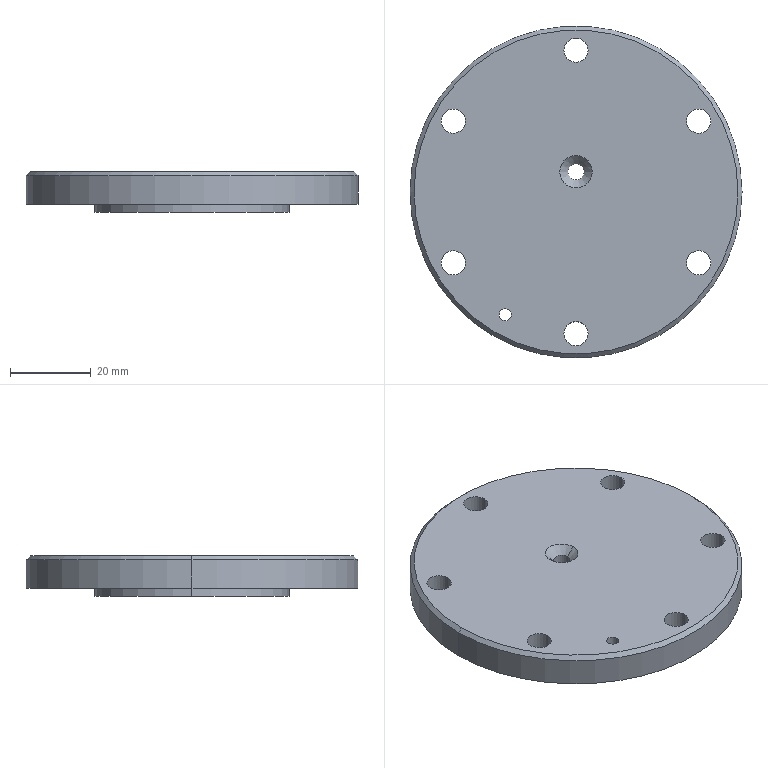Part | SolidWorks | features Chamfer 2, ICE 1, Revolution 1 | 1 solid | 27 faces | box 82 x 82 x 10 mm | volume 44167 mm3 | cylinder 20 | cone 4 | plane 3 | commonest cylinder face diameters 6 x12 3 x2 4 x2 48 x2 82 x2
STEP:
#1=CARTESIAN_POINT('',(-2.,5.,8.));
#2=VERTEX_POINT('',#1);
#3=CARTESIAN_POINT('',(2.,5.,8.));
#4=VERTEX_POINT('',#3);
#5=CARTESIAN_POINT('',(0.,5.,8.));
#6=DIRECTION('',(0.,0.,1.));
#7=DIRECTION('',(-1.,0.,0.));
#8=AXIS2_PLACEMENT_3D('',#5,#6,#7);
#9=CIRCLE('',#8,2.);
#10=EDGE_CURVE('',#2,#4,#9,.T.);
#11=ORIENTED_EDGE('',*,*,#10,.F.);
#12=CARTESIAN_POINT('',(-4.,5.,10.));
#13=VERTEX_POINT('',#12);
#14=CARTESIAN_POINT('',(-4.,5.,10.));
#15=DIRECTION('',(-0.7071,0.,0.7071));
#16=VECTOR('',#15,1000.);
#17=LINE('',#14,#16);
#18=EDGE_CURVE('',#2,#13,#17,.T.);
#19=ORIENTED_EDGE('',*,*,#18,.T.);
#20=CARTESIAN_POINT('',(4.,5.,10.));
#21=VERTEX_POINT('',#20);
#22=CARTESIAN_POINT('',(0.,5.,10.));
#23=DIRECTION('',(0.,0.,-1.));
#24=DIRECTION('',(-1.,0.,0.));
#25=AXIS2_PLACEMENT_3D('',#22,#23,#24);
#26=CIRCLE('',#25,4.);
#27=EDGE_CURVE('',#21,#13,#26,.T.);
#28=ORIENTED_EDGE('',*,*,#27,.F.);
#29=CARTESIAN_POINT('',(4.,5.,10.));
#30=DIRECTION('',(0.7071,0.,0.7071));
#31=VECTOR('',#30,1000.);
#32=LINE('',#29,#31);
#33=EDGE_CURVE('',#4,#21,#32,.T.);
#34=ORIENTED_EDGE('',*,*,#33,.F.);
#35=EDGE_LOOP('',(#11,#19,#28,#34));
#36=FACE_OUTER_BOUND('',#35,.T.);
#37=CARTESIAN_POINT('',(0.,5.,10.));
#38=DIRECTION('',(0.,0.,1.));
#39=DIRECTION('',(1.,0.,0.));
#40=AXIS2_PLACEMENT_3D('',#37,#38,#39);
#41=CONICAL_SURFACE('',#40,4.,0.7854);
#42=ADVANCED_FACE('',(#36),#41,.F.);
#43=CARTESIAN_POINT('',(40.,0.,10.));
#44=VERTEX_POINT('',#43);
#45=CARTESIAN_POINT('',(-40.,0.,10.));
#46=VERTEX_POINT('',#45);
#47=CARTESIAN_POINT('',(0.,0.,10.));
#48=DIRECTION('',(0.,0.,1.));
#49=DIRECTION('',(-1.,0.,0.));
#50=AXIS2_PLACEMENT_3D('',#47,#48,#49);
#51=CIRCLE('',#50,40.);
#52=EDGE_CURVE('',#44,#46,#51,.T.);
#53=ORIENTED_EDGE('',*,*,#52,.F.);
#54=CARTESIAN_POINT('',(41.,0.,9.));
#55=VERTEX_POINT('',#54);
#56=CARTESIAN_POINT('',(40.,0.,10.));
#57=DIRECTION('',(0.7071,0.,-0.7071));
#58=VECTOR('',#57,1000.);
#59=LINE('',#56,#58);
#60=EDGE_CURVE('',#44,#55,#59,.T.);
#61=ORIENTED_EDGE('',*,*,#60,.T.);
#62=CARTESIAN_POINT('',(-41.,0.,9.));
#63=VERTEX_POINT('',#62);
#64=CARTESIAN_POINT('',(0.,0.,9.));
#65=DIRECTION('',(0.,0.,-1.));
#66=DIRECTION('',(-1.,0.,0.));
#67=AXIS2_PLACEMENT_3D('',#64,#65,#66);
#68=CIRCLE('',#67,41.);
#69=EDGE_CURVE('',#63,#55,#68,.T.);
#70=ORIENTED_EDGE('',*,*,#69,.F.);
#71=CARTESIAN_POINT('',(-40.,0.,10.));
#72=DIRECTION('',(-0.7071,0.,-0.7071));
#73=VECTOR('',#72,1000.);
#74=LINE('',#71,#73);
#75=EDGE_CURVE('',#46,#63,#74,.T.);
#76=ORIENTED_EDGE('',*,*,#75,.F.);
#77=EDGE_LOOP('',(#53,#61,#70,#76));
#78=FACE_OUTER_BOUND('',#77,.T.);
#79=CARTESIAN_POINT('',(0.,0.,10.));
#80=DIRECTION('',(0.,0.,-1.));
#81=DIRECTION('',(-1.,0.,0.));
#82=AXIS2_PLACEMENT_3D('',#79,#80,#81);
#83=CONICAL_SURFACE('',#82,40.,0.7854);
#84=ADVANCED_FACE('',(#78),#83,.T.);
#85=CARTESIAN_POINT('',(3.,35.,2.));
#86=VERTEX_POINT('',#85);
#87=CARTESIAN_POINT('',(-3.,35.,2.));
#88=VERTEX_POINT('',#87);
#89=CARTESIAN_POINT('',(0.,35.,2.));
#90=DIRECTION('',(0.,0.,-1.));
#91=DIRECTION('',(1.,0.,0.));
#92=AXIS2_PLACEMENT_3D('',#89,#90,#91);
#93=CIRCLE('',#92,3.);
#94=EDGE_CURVE('',#86,#88,#93,.T.);
#95=ORIENTED_EDGE('',*,*,#94,.T.);
#96=CARTESIAN_POINT('',(-3.,35.,10.));
#97=VERTEX_POINT('',#96);
#98=CARTESIAN_POINT('',(-3.,35.,-8.));
#99=DIRECTION('',(0.,0.,1.));
#100=VECTOR('',#99,1000.);
#101=LINE('',#98,#100);
#102=EDGE_CURVE('',#88,#97,#101,.T.);
#103=ORIENTED_EDGE('',*,*,#102,.T.);
#104=CARTESIAN_POINT('',(3.,35.,10.));
#105=VERTEX_POINT('',#104);
#106=CARTESIAN_POINT('',(0.,35.,10.));
#107=DIRECTION('',(0.,0.,-1.));
#108=DIRECTION('',(-1.,0.,0.));
#109=AXIS2_PLACEMENT_3D('',#106,#107,#108);
#110=CIRCLE('',#109,3.);
#111=EDGE_CURVE('',#105,#97,#110,.T.);
#112=ORIENTED_EDGE('',*,*,#111,.F.);
#113=CARTESIAN_POINT('',(3.,35.,-8.));
#114=DIRECTION('',(0.,0.,1.));
#115=VECTOR('',#114,1000.);
#116=LINE('',#113,#115);
#117=EDGE_CURVE('',#86,#105,#116,.T.);
#118=ORIENTED_EDGE('',*,*,#117,.F.);
#119=EDGE_LOOP('',(#95,#103,#112,#118));
#120=FACE_OUTER_BOUND('',#119,.T.);
#121=CARTESIAN_POINT('',(0.,35.,-8.));
#122=DIRECTION('',(0.,0.,1.));
#123=DIRECTION('',(1.,0.,0.));
#124=AXIS2_PLACEMENT_3D('',#121,#122,#123);
#125=CYLINDRICAL_SURFACE('',#124,3.);
#126=ADVANCED_FACE('',(#120),#125,.F.);
#127=CARTESIAN_POINT('',(33.311,17.5,2.));
#128=VERTEX_POINT('',#127);
#129=CARTESIAN_POINT('',(27.311,17.5,2.));
#130=VERTEX_POINT('',#129);
#131=CARTESIAN_POINT('',(30.311,17.5,2.));
#132=DIRECTION('',(0.,0.,-1.));
#133=DIRECTION('',(1.,0.,0.));
#134=AXIS2_PLACEMENT_3D('',#131,#132,#133);
#135=CIRCLE('',#134,3.);
#136=EDGE_CURVE('',#128,#130,#135,.T.);
#137=ORIENTED_EDGE('',*,*,#136,.T.);
#138=CARTESIAN_POINT('',(27.311,17.5,10.));
#139=VERTEX_POINT('',#138);
#140=CARTESIAN_POINT('',(27.311,17.5,-8.));
#141=DIRECTION('',(0.,0.,1.));
#142=VECTOR('',#141,1000.);
#143=LINE('',#140,#142);
#144=EDGE_CURVE('',#130,#139,#143,.T.);
#145=ORIENTED_EDGE('',*,*,#144,.T.);
#146=CARTESIAN_POINT('',(33.311,17.5,10.));
#147=VERTEX_POINT('',#146);
#148=CARTESIAN_POINT('',(30.311,17.5,10.));
#149=DIRECTION('',(0.,0.,-1.));
#150=DIRECTION('',(-1.,0.,0.));
#151=AXIS2_PLACEMENT_3D('',#148,#149,#150);
#152=CIRCLE('',#151,3.);
#153=EDGE_CURVE('',#147,#139,#152,.T.);
#154=ORIENTED_EDGE('',*,*,#153,.F.);
#155=CARTESIAN_POINT('',(33.311,17.5,-8.));
#156=DIRECTION('',(0.,0.,1.));
#157=VECTOR('',#156,1000.);
#158=LINE('',#155,#157);
#159=EDGE_CURVE('',#128,#147,#158,.T.);
#160=ORIENTED_EDGE('',*,*,#159,.F.);
#161=EDGE_LOOP('',(#137,#145,#154,#160));
#162=FACE_OUTER_BOUND('',#161,.T.);
#163=CARTESIAN_POINT('',(30.311,17.5,-8.));
#164=DIRECTION('',(0.,0.,1.));
#165=DIRECTION('',(1.,0.,0.));
#166=AXIS2_PLACEMENT_3D('',#163,#164,#165);
#167=CYLINDRICAL_SURFACE('',#166,3.);
#168=ADVANCED_FACE('',(#162),#167,.F.);
#169=CARTESIAN_POINT('',(-16.,-30.311,2.));
#170=VERTEX_POINT('',#169);
#171=CARTESIAN_POINT('',(-19.,-30.311,2.));
#172=VERTEX_POINT('',#171);
#173=CARTESIAN_POINT('',(-17.5,-30.311,2.));
#174=DIRECTION('',(0.,0.,-1.));
#175=DIRECTION('',(1.,0.,0.));
#176=AXIS2_PLACEMENT_3D('',#173,#174,#175);
#177=CIRCLE('',#176,1.5);
#178=EDGE_CURVE('',#170,#172,#177,.T.);
#179=ORIENTED_EDGE('',*,*,#178,.T.);
#180=CARTESIAN_POINT('',(-19.,-30.311,10.));
#181=VERTEX_POINT('',#180);
#182=CARTESIAN_POINT('',(-19.,-30.311,-8.));
#183=DIRECTION('',(0.,0.,1.));
#184=VECTOR('',#183,1000.);
#185=LINE('',#182,#184);
#186=EDGE_CURVE('',#172,#181,#185,.T.);
#187=ORIENTED_EDGE('',*,*,#186,.T.);
#188=CARTESIAN_POINT('',(-16.,-30.311,10.));
#189=VERTEX_POINT('',#188);
#190=CARTESIAN_POINT('',(-17.5,-30.311,10.));
#191=DIRECTION('',(0.,0.,-1.));
#192=DIRECTION('',(-1.,0.,0.));
#193=AXIS2_PLACEMENT_3D('',#190,#191,#192);
#194=CIRCLE('',#193,1.5);
#195=EDGE_CURVE('',#189,#181,#194,.T.);
#196=ORIENTED_EDGE('',*,*,#195,.F.);
#197=CARTESIAN_POINT('',(-16.,-30.311,-8.));
#198=DIRECTION('',(0.,0.,1.));
#199=VECTOR('',#198,1000.);
#200=LINE('',#197,#199);
#201=EDGE_CURVE('',#170,#189,#200,.T.);
#202=ORIENTED_EDGE('',*,*,#201,.F.);
#203=EDGE_LOOP('',(#179,#187,#196,#202));
#204=FACE_OUTER_BOUND('',#203,.T.);
#205=CARTESIAN_POINT('',(-17.5,-30.311,-8.));
#206=DIRECTION('',(0.,0.,1.));
#207=DIRECTION('',(1.,0.,0.));
#208=AXIS2_PLACEMENT_3D('',#205,#206,#207);
#209=CYLINDRICAL_SURFACE('',#208,1.5);
#210=ADVANCED_FACE('',(#204),#209,.F.);
#211=CARTESIAN_POINT('',(2.,5.,0.));
#212=VERTEX_POINT('',#211);
#213=CARTESIAN_POINT('',(-2.,5.,0.));
#214=VERTEX_POINT('',#213);
#215=CARTESIAN_POINT('',(0.,5.,0.));
#216=DIRECTION('',(0.,0.,-1.));
#217=DIRECTION('',(1.,0.,0.));
#218=AXIS2_PLACEMENT_3D('',#215,#216,#217);
#219=CIRCLE('',#218,2.);
#220=EDGE_CURVE('',#212,#214,#219,.T.);
#221=ORIENTED_EDGE('',*,*,#220,.T.);
#222=CARTESIAN_POINT('',(-2.,5.,-8.));
#223=DIRECTION('',(0.,0.,1.));
#224=VECTOR('',#223,1000.);
#225=LINE('',#222,#224);
#226=EDGE_CURVE('',#214,#2,#225,.T.);
#227=ORIENTED_EDGE('',*,*,#226,.T.);
#228=ORIENTED_EDGE('',*,*,#10,.T.);
#229=CARTESIAN_POINT('',(2.,5.,-8.));
#230=DIRECTION('',(0.,0.,1.));
#231=VECTOR('',#230,1000.);
#232=LINE('',#229,#231);
#233=EDGE_CURVE('',#212,#4,#232,.T.);
#234=ORIENTED_EDGE('',*,*,#233,.F.);
#235=EDGE_LOOP('',(#221,#227,#228,#234));
#236=FACE_OUTER_BOUND('',#235,.T.);
#237=CARTESIAN_POINT('',(0.,5.,-8.));
#238=DIRECTION('',(0.,0.,1.));
#239=DIRECTION('',(1.,0.,0.));
#240=AXIS2_PLACEMENT_3D('',#237,#238,#239);
#241=CYLINDRICAL_SURFACE('',#240,2.);
#242=ADVANCED_FACE('',(#236),#241,.F.);
#243=CARTESIAN_POINT('',(33.311,-17.5,2.));
#244=VERTEX_POINT('',#243);
#245=CARTESIAN_POINT('',(27.311,-17.5,2.));
#246=VERTEX_POINT('',#245);
#247=CARTESIAN_POINT('',(30.311,-17.5,2.));
#248=DIRECTION('',(0.,0.,-1.));
#249=DIRECTION('',(1.,0.,0.));
#250=AXIS2_PLACEMENT_3D('',#247,#248,#249);
#251=CIRCLE('',#250,3.);
#252=EDGE_CURVE('',#244,#246,#251,.T.);
#253=ORIENTED_EDGE('',*,*,#252,.T.);
#254=CARTESIAN_POINT('',(27.311,-17.5,10.));
#255=VERTEX_POINT('',#254);
#256=CARTESIAN_POINT('',(27.311,-17.5,-8.));
#257=DIRECTION('',(0.,0.,1.));
#258=VECTOR('',#257,1000.);
#259=LINE('',#256,#258);
#260=EDGE_CURVE('',#246,#255,#259,.T.);
#261=ORIENTED_EDGE('',*,*,#260,.T.);
#262=CARTESIAN_POINT('',(33.311,-17.5,10.));
#263=VERTEX_POINT('',#262);
#264=CARTESIAN_POINT('',(30.311,-17.5,10.));
#265=DIRECTION('',(0.,0.,-1.));
#266=DIRECTION('',(-1.,0.,0.));
#267=AXIS2_PLACEMENT_3D('',#264,#265,#266);
#268=CIRCLE('',#267,3.);
#269=EDGE_CURVE('',#263,#255,#268,.T.);
#270=ORIENTED_EDGE('',*,*,#269,.F.);
#271=CARTESIAN_POINT('',(33.311,-17.5,-8.));
#272=DIRECTION('',(0.,0.,1.));
#273=VECTOR('',#272,1000.);
#274=LINE('',#271,#273);
#275=EDGE_CURVE('',#244,#263,#274,.T.);
#276=ORIENTED_EDGE('',*,*,#275,.F.);
#277=EDGE_LOOP('',(#253,#261,#270,#276));
#278=FACE_OUTER_BOUND('',#277,.T.);
#279=CARTESIAN_POINT('',(30.311,-17.5,-8.));
#280=DIRECTION('',(0.,0.,1.));
#281=DIRECTION('',(1.,0.,0.));
#282=AXIS2_PLACEMENT_3D('',#279,#280,#281);
#283=CYLINDRICAL_SURFACE('',#282,3.);
#284=ADVANCED_FACE('',(#278),#283,.F.);
#285=CARTESIAN_POINT('',(3.,-35.,2.));
#286=VERTEX_POINT('',#285);
#287=CARTESIAN_POINT('',(-3.,-35.,2.));
#288=VERTEX_POINT('',#287);
#289=CARTESIAN_POINT('',(0.,-35.,2.));
#290=DIRECTION('',(0.,0.,-1.));
#291=DIRECTION('',(1.,0.,0.));
#292=AXIS2_PLACEMENT_3D('',#289,#290,#291);
#293=CIRCLE('',#292,3.);
#294=EDGE_CURVE('',#286,#288,#293,.T.);
#295=ORIENTED_EDGE('',*,*,#294,.T.);
#296=CARTESIAN_POINT('',(-3.,-35.,10.));
#297=VERTEX_POINT('',#296);
#298=CARTESIAN_POINT('',(-3.,-35.,-8.));
#299=DIRECTION('',(0.,0.,1.));
#300=VECTOR('',#299,1000.);
#301=LINE('',#298,#300);
#302=EDGE_CURVE('',#288,#297,#301,.T.);
#303=ORIENTED_EDGE('',*,*,#302,.T.);
#304=CARTESIAN_POINT('',(3.,-35.,10.));
#305=VERTEX_POINT('',#304);
#306=CARTESIAN_POINT('',(0.,-35.,10.));
#307=DIRECTION('',(0.,0.,-1.));
#308=DIRECTION('',(-1.,0.,0.));
#309=AXIS2_PLACEMENT_3D('',#306,#307,#308);
#310=CIRCLE('',#309,3.);
#311=EDGE_CURVE('',#305,#297,#310,.T.);
#312=ORIENTED_EDGE('',*,*,#311,.F.);
#313=CARTESIAN_POINT('',(3.,-35.,-8.));
#314=DIRECTION('',(0.,0.,1.));
#315=VECTOR('',#314,1000.);
#316=LINE('',#313,#315);
#317=EDGE_CURVE('',#286,#305,#316,.T.);
#318=ORIENTED_EDGE('',*,*,#317,.F.);
#319=EDGE_LOOP('',(#295,#303,#312,#318));
#320=FACE_OUTER_BOUND('',#319,.T.);
#321=CARTESIAN_POINT('',(0.,-35.,-8.));
#322=DIRECTION('',(0.,0.,1.));
#323=DIRECTION('',(1.,0.,0.));
#324=AXIS2_PLACEMENT_3D('',#321,#322,#323);
#325=CYLINDRICAL_SURFACE('',#324,3.);
#326=ADVANCED_FACE('',(#320),#325,.F.);
#327=CARTESIAN_POINT('',(-27.311,-17.5,2.));
#328=VERTEX_POINT('',#327);
#329=CARTESIAN_POINT('',(-33.311,-17.5,2.));
#330=VERTEX_POINT('',#329);
#331=CARTESIAN_POINT('',(-30.311,-17.5,2.));
#332=DIRECTION('',(0.,0.,-1.));
#333=DIRECTION('',(1.,0.,0.));
#334=AXIS2_PLACEMENT_3D('',#331,#332,#333);
#335=CIRCLE('',#334,3.);
#336=EDGE_CURVE('',#328,#330,#335,.T.);
#337=ORIENTED_EDGE('',*,*,#336,.T.);
#338=CARTESIAN_POINT('',(-33.311,-17.5,10.));
#339=VERTEX_POINT('',#338);
#340=CARTESIAN_POINT('',(-33.311,-17.5,-8.));
#341=DIRECTION('',(0.,0.,1.));
#342=VECTOR('',#341,1000.);
#343=LINE('',#340,#342);
#344=EDGE_CURVE('',#330,#339,#343,.T.);
#345=ORIENTED_EDGE('',*,*,#344,.T.);
#346=CARTESIAN_POINT('',(-27.311,-17.5,10.));
#347=VERTEX_POINT('',#346);
#348=CARTESIAN_POINT('',(-30.311,-17.5,10.));
#349=DIRECTION('',(0.,0.,-1.));
#350=DIRECTION('',(-1.,0.,0.));
#351=AXIS2_PLACEMENT_3D('',#348,#349,#350);
#352=CIRCLE('',#351,3.);
#353=EDGE_CURVE('',#347,#339,#352,.T.);
#354=ORIENTED_EDGE('',*,*,#353,.F.);
#355=CARTESIAN_POINT('',(-27.311,-17.5,-8.));
#356=DIRECTION('',(0.,0.,1.));
#357=VECTOR('',#356,1000.);
#358=LINE('',#355,#357);
#359=EDGE_CURVE('',#328,#347,#358,.T.);
#360=ORIENTED_EDGE('',*,*,#359,.F.);
#361=EDGE_LOOP('',(#337,#345,#354,#360));
#362=FACE_OUTER_BOUND('',#361,.T.);
#363=CARTESIAN_POINT('',(-30.311,-17.5,-8.));
#364=DIRECTION('',(0.,0.,1.));
#365=DIRECTION('',(1.,0.,0.));
#366=AXIS2_PLACEMENT_3D('',#363,#364,#365);
#367=CYLINDRICAL_SURFACE('',#366,3.);
#368=ADVANCED_FACE('',(#362),#367,.F.);
#369=CARTESIAN_POINT('',(-27.311,17.5,2.));
#370=VERTEX_POINT('',#369);
#371=CARTESIAN_POINT('',(-33.311,17.5,2.));
#372=VERTEX_POINT('',#371);
#373=CARTESIAN_POINT('',(-30.311,17.5,2.));
#374=DIRECTION('',(0.,0.,-1.));
#375=DIRECTION('',(1.,0.,0.));
#376=AXIS2_PLACEMENT_3D('',#373,#374,#375);
#377=CIRCLE('',#376,3.);
#378=EDGE_CURVE('',#370,#372,#377,.T.);
#379=ORIENTED_EDGE('',*,*,#378,.T.);
#380=CARTESIAN_POINT('',(-33.311,17.5,10.));
#381=VERTEX_POINT('',#380);
#382=CARTESIAN_POINT('',(-33.311,17.5,-8.));
#383=DIRECTION('',(0.,0.,1.));
#384=VECTOR('',#383,1000.);
#385=LINE('',#382,#384);
#386=EDGE_CURVE('',#372,#381,#385,.T.);
#387=ORIENTED_EDGE('',*,*,#386,.T.);
#388=CARTESIAN_POINT('',(-27.311,17.5,10.));
#389=VERTEX_POINT('',#388);
#390=CARTESIAN_POINT('',(-30.311,17.5,10.));
#391=DIRECTION('',(0.,0.,-1.));
#392=DIRECTION('',(-1.,0.,0.));
#393=AXIS2_PLACEMENT_3D('',#390,#391,#392);
#394=CIRCLE('',#393,3.);
#395=EDGE_CURVE('',#389,#381,#394,.T.);
#396=ORIENTED_EDGE('',*,*,#395,.F.);
#397=CARTESIAN_POINT('',(-27.311,17.5,-8.));
#398=DIRECTION('',(0.,0.,1.));
#399=VECTOR('',#398,1000.);
#400=LINE('',#397,#399);
#401=EDGE_CURVE('',#370,#389,#400,.T.);
#402=ORIENTED_EDGE('',*,*,#401,.F.);
#403=EDGE_LOOP('',(#379,#387,#396,#402));
#404=FACE_OUTER_BOUND('',#403,.T.);
#405=CARTESIAN_POINT('',(-30.311,17.5,-8.));
#406=DIRECTION('',(0.,0.,1.));
#407=DIRECTION('',(1.,0.,0.));
#408=AXIS2_PLACEMENT_3D('',#405,#406,#407);
#409=CYLINDRICAL_SURFACE('',#408,3.);
#410=ADVANCED_FACE('',(#404),#409,.F.);
#411=CARTESIAN_POINT('',(41.,0.,2.));
#412=VERTEX_POINT('',#411);
#413=CARTESIAN_POINT('',(-41.,0.,2.));
#414=VERTEX_POINT('',#413);
#415=CARTESIAN_POINT('',(0.,0.,2.));
#416=DIRECTION('',(0.,0.,1.));
#417=DIRECTION('',(1.,0.,0.));
#418=AXIS2_PLACEMENT_3D('',#415,#416,#417);
#419=CIRCLE('',#418,41.);
#420=EDGE_CURVE('',#412,#414,#419,.T.);
#421=ORIENTED_EDGE('',*,*,#420,.T.);
#422=CARTESIAN_POINT('',(-41.,0.,25.938));
#423=DIRECTION('',(0.,0.,1.));
#424=VECTOR('',#423,1000.);
#425=LINE('',#422,#424);
#426=EDGE_CURVE('',#414,#63,#425,.T.);
#427=ORIENTED_EDGE('',*,*,#426,.T.);
#428=ORIENTED_EDGE('',*,*,#69,.T.);
#429=CARTESIAN_POINT('',(41.,0.,25.938));
#430=DIRECTION('',(0.,0.,1.));
#431=VECTOR('',#430,1000.);
#432=LINE('',#429,#431);
#433=EDGE_CURVE('',#412,#55,#432,.T.);
#434=ORIENTED_EDGE('',*,*,#433,.F.);
#435=EDGE_LOOP('',(#421,#427,#428,#434));
#436=FACE_OUTER_BOUND('',#435,.T.);
#437=CARTESIAN_POINT('',(0.,0.,25.938));
#438=DIRECTION('',(0.,0.,1.));
#439=DIRECTION('',(1.,0.,0.));
#440=AXIS2_PLACEMENT_3D('',#437,#438,#439);
#441=CYLINDRICAL_SURFACE('',#440,41.);
#442=ADVANCED_FACE('',(#436),#441,.T.);
#443=CARTESIAN_POINT('',(24.,0.,0.));
#444=VERTEX_POINT('',#443);
#445=CARTESIAN_POINT('',(-24.,0.,0.));
#446=VERTEX_POINT('',#445);
#447=CARTESIAN_POINT('',(0.,0.,0.));
#448=DIRECTION('',(0.,0.,1.));
#449=DIRECTION('',(1.,0.,0.));
#450=AXIS2_PLACEMENT_3D('',#447,#448,#449);
#451=CIRCLE('',#450,24.);
#452=EDGE_CURVE('',#444,#446,#451,.T.);
#453=ORIENTED_EDGE('',*,*,#452,.T.);
#454=CARTESIAN_POINT('',(-24.,0.,2.));
#455=VERTEX_POINT('',#454);
#456=CARTESIAN_POINT('',(-24.,0.,25.938));
#457=DIRECTION('',(0.,0.,1.));
#458=VECTOR('',#457,1000.);
#459=LINE('',#456,#458);
#460=EDGE_CURVE('',#446,#455,#459,.T.);
#461=ORIENTED_EDGE('',*,*,#460,.T.);
#462=CARTESIAN_POINT('',(24.,0.,2.));
#463=VERTEX_POINT('',#462);
#464=CARTESIAN_POINT('',(0.,0.,2.));
#465=DIRECTION('',(0.,0.,1.));
#466=DIRECTION('',(1.,0.,0.));
#467=AXIS2_PLACEMENT_3D('',#464,#465,#466);
#468=CIRCLE('',#467,24.);
#469=EDGE_CURVE('',#463,#455,#468,.T.);
#470=ORIENTED_EDGE('',*,*,#469,.F.);
#471=CARTESIAN_POINT('',(24.,0.,25.938));
#472=DIRECTION('',(0.,0.,1.));
#473=VECTOR('',#472,1000.);
#474=LINE('',#471,#473);
#475=EDGE_CURVE('',#444,#463,#474,.T.);
#476=ORIENTED_EDGE('',*,*,#475,.F.);
#477=EDGE_LOOP('',(#453,#461,#470,#476));
#478=FACE_OUTER_BOUND('',#477,.T.);
#479=CARTESIAN_POINT('',(0.,0.,25.938));
#480=DIRECTION('',(0.,0.,1.));
#481=DIRECTION('',(1.,0.,0.));
#482=AXIS2_PLACEMENT_3D('',#479,#480,#481);
#483=CYLINDRICAL_SURFACE('',#482,24.);
#484=ADVANCED_FACE('',(#478),#483,.T.);
#485=ORIENTED_EDGE('',*,*,#220,.F.);
#486=CARTESIAN_POINT('',(0.,5.,0.));
#487=DIRECTION('',(0.,0.,-1.));
#488=DIRECTION('',(1.,0.,0.));
#489=AXIS2_PLACEMENT_3D('',#486,#487,#488);
#490=CIRCLE('',#489,2.);
#491=EDGE_CURVE('',#214,#212,#490,.T.);
#492=ORIENTED_EDGE('',*,*,#491,.F.);
#493=EDGE_LOOP('',(#485,#492));
#494=FACE_BOUND('',#493,.T.);
#495=ORIENTED_EDGE('',*,*,#452,.F.);
#496=CARTESIAN_POINT('',(0.,0.,0.));
#497=DIRECTION('',(0.,0.,1.));
#498=DIRECTION('',(1.,0.,0.));
#499=AXIS2_PLACEMENT_3D('',#496,#497,#498);
#500=CIRCLE('',#499,24.);
#501=EDGE_CURVE('',#446,#444,#500,.T.);
#502=ORIENTED_EDGE('',*,*,#501,.F.);
#503=EDGE_LOOP('',(#495,#502));
#504=FACE_OUTER_BOUND('',#503,.T.);
#505=CARTESIAN_POINT('',(0.,0.,0.));
#506=DIRECTION('',(0.,0.,1.));
#507=DIRECTION('',(1.,0.,0.));
#508=AXIS2_PLACEMENT_3D('',#505,#506,#507);
#509=PLANE('',#508);
#510=ADVANCED_FACE('',(#494,#504),#509,.F.);
#511=ORIENTED_EDGE('',*,*,#460,.F.);
#512=ORIENTED_EDGE('',*,*,#501,.T.);
#513=ORIENTED_EDGE('',*,*,#475,.T.);
#514=CARTESIAN_POINT('',(0.,0.,2.));
#515=DIRECTION('',(0.,0.,1.));
#516=DIRECTION('',(1.,0.,0.));
#517=AXIS2_PLACEMENT_3D('',#514,#515,#516);
#518=CIRCLE('',#517,24.);
#519=EDGE_CURVE('',#455,#463,#518,.T.);
#520=ORIENTED_EDGE('',*,*,#519,.F.);
#521=EDGE_LOOP('',(#511,#512,#513,#520));
#522=FACE_OUTER_BOUND('',#521,.T.);
#523=CARTESIAN_POINT('',(0.,0.,25.938));
#524=DIRECTION('',(0.,0.,1.));
#525=DIRECTION('',(1.,0.,0.));
#526=AXIS2_PLACEMENT_3D('',#523,#524,#525);
#527=CYLINDRICAL_SURFACE('',#526,24.);
#528=ADVANCED_FACE('',(#522),#527,.T.);
#529=ORIENTED_EDGE('',*,*,#94,.F.);
#530=CARTESIAN_POINT('',(0.,35.,2.));
#531=DIRECTION('',(0.,0.,-1.));
#532=DIRECTION('',(1.,0.,0.));
#533=AXIS2_PLACEMENT_3D('',#530,#531,#532);
#534=CIRCLE('',#533,3.);
#535=EDGE_CURVE('',#88,#86,#534,.T.);
#536=ORIENTED_EDGE('',*,*,#535,.F.);
#537=EDGE_LOOP('',(#529,#536));
#538=FACE_BOUND('',#537,.T.);
#539=ORIENTED_EDGE('',*,*,#136,.F.);
#540=CARTESIAN_POINT('',(30.311,17.5,2.));
#541=DIRECTION('',(0.,0.,-1.));
#542=DIRECTION('',(1.,0.,0.));
#543=AXIS2_PLACEMENT_3D('',#540,#541,#542);
#544=CIRCLE('',#543,3.);
#545=EDGE_CURVE('',#130,#128,#544,.T.);
#546=ORIENTED_EDGE('',*,*,#545,.F.);
#547=EDGE_LOOP('',(#539,#546));
#548=FACE_BOUND('',#547,.T.);
#549=ORIENTED_EDGE('',*,*,#178,.F.);
#550=CARTESIAN_POINT('',(-17.5,-30.311,2.));
#551=DIRECTION('',(0.,0.,-1.));
#552=DIRECTION('',(1.,0.,0.));
#553=AXIS2_PLACEMENT_3D('',#550,#551,#552);
#554=CIRCLE('',#553,1.5);
#555=EDGE_CURVE('',#172,#170,#554,.T.);
#556=ORIENTED_EDGE('',*,*,#555,.F.);
#557=EDGE_LOOP('',(#549,#556));
#558=FACE_BOUND('',#557,.T.);
#559=ORIENTED_EDGE('',*,*,#252,.F.);
#560=CARTESIAN_POINT('',(30.311,-17.5,2.));
#561=DIRECTION('',(0.,0.,-1.));
#562=DIRECTION('',(1.,0.,0.));
#563=AXIS2_PLACEMENT_3D('',#560,#561,#562);
#564=CIRCLE('',#563,3.);
#565=EDGE_CURVE('',#246,#244,#564,.T.);
#566=ORIENTED_EDGE('',*,*,#565,.F.);
#567=EDGE_LOOP('',(#559,#566));
#568=FACE_BOUND('',#567,.T.);
#569=ORIENTED_EDGE('',*,*,#294,.F.);
#570=CARTESIAN_POINT('',(0.,-35.,2.));
#571=DIRECTION('',(0.,0.,-1.));
#572=DIRECTION('',(1.,0.,0.));
#573=AXIS2_PLACEMENT_3D('',#570,#571,#572);
#574=CIRCLE('',#573,3.);
#575=EDGE_CURVE('',#288,#286,#574,.T.);
#576=ORIENTED_EDGE('',*,*,#575,.F.);
#577=EDGE_LOOP('',(#569,#576));
#578=FACE_BOUND('',#577,.T.);
#579=ORIENTED_EDGE('',*,*,#336,.F.);
#580=CARTESIAN_POINT('',(-30.311,-17.5,2.));
#581=DIRECTION('',(0.,0.,-1.));
#582=DIRECTION('',(1.,0.,0.));
#583=AXIS2_PLACEMENT_3D('',#580,#581,#582);
#584=CIRCLE('',#583,3.);
#585=EDGE_CURVE('',#330,#328,#584,.T.);
#586=ORIENTED_EDGE('',*,*,#585,.F.);
#587=EDGE_LOOP('',(#579,#586));
#588=FACE_BOUND('',#587,.T.);
#589=ORIENTED_EDGE('',*,*,#378,.F.);
#590=CARTESIAN_POINT('',(-30.311,17.5,2.));
#591=DIRECTION('',(0.,0.,-1.));
#592=DIRECTION('',(1.,0.,0.));
#593=AXIS2_PLACEMENT_3D('',#590,#591,#592);
#594=CIRCLE('',#593,3.);
#595=EDGE_CURVE('',#372,#370,#594,.T.);
#596=ORIENTED_EDGE('',*,*,#595,.F.);
#597=EDGE_LOOP('',(#589,#596));
#598=FACE_BOUND('',#597,.T.);
#599=ORIENTED_EDGE('',*,*,#420,.F.);
#600=CARTESIAN_POINT('',(0.,0.,2.));
#601=DIRECTION('',(0.,0.,1.));
#602=DIRECTION('',(1.,0.,0.));
#603=AXIS2_PLACEMENT_3D('',#600,#601,#602);
#604=CIRCLE('',#603,41.);
#605=EDGE_CURVE('',#414,#412,#604,.T.);
#606=ORIENTED_EDGE('',*,*,#605,.F.);
#607=EDGE_LOOP('',(#599,#606));
#608=FACE_OUTER_BOUND('',#607,.T.);
#609=ORIENTED_EDGE('',*,*,#469,.T.);
#610=ORIENTED_EDGE('',*,*,#519,.T.);
#611=EDGE_LOOP('',(#609,#610));
#612=FACE_BOUND('',#611,.T.);
#613=CARTESIAN_POINT('',(0.,24.,2.));
#614=DIRECTION('',(0.,0.,1.));
#615=DIRECTION('',(1.,0.,0.));
#616=AXIS2_PLACEMENT_3D('',#613,#614,#615);
#617=PLANE('',#616);
#618=ADVANCED_FACE('',(#538,#548,#558,#568,#578,#588,#598,#608,#612),#617,.F.);
#619=ORIENTED_EDGE('',*,*,#426,.F.);
#620=ORIENTED_EDGE('',*,*,#605,.T.);
#621=ORIENTED_EDGE('',*,*,#433,.T.);
#622=CARTESIAN_POINT('',(0.,0.,9.));
#623=DIRECTION('',(0.,0.,-1.));
#624=DIRECTION('',(-1.,0.,0.));
#625=AXIS2_PLACEMENT_3D('',#622,#623,#624);
#626=CIRCLE('',#625,41.);
#627=EDGE_CURVE('',#55,#63,#626,.T.);
#628=ORIENTED_EDGE('',*,*,#627,.T.);
#629=EDGE_LOOP('',(#619,#620,#621,#628));
#630=FACE_OUTER_BOUND('',#629,.T.);
#631=CARTESIAN_POINT('',(0.,0.,25.938));
#632=DIRECTION('',(0.,0.,1.));
#633=DIRECTION('',(1.,0.,0.));
#634=AXIS2_PLACEMENT_3D('',#631,#632,#633);
#635=CYLINDRICAL_SURFACE('',#634,41.);
#636=ADVANCED_FACE('',(#630),#635,.T.);
#637=ORIENTED_EDGE('',*,*,#27,.T.);
#638=CARTESIAN_POINT('',(0.,5.,10.));
#639=DIRECTION('',(0.,0.,-1.));
#640=DIRECTION('',(-1.,0.,0.));
#641=AXIS2_PLACEMENT_3D('',#638,#639,#640);
#642=CIRCLE('',#641,4.);
#643=EDGE_CURVE('',#13,#21,#642,.T.);
#644=ORIENTED_EDGE('',*,*,#643,.T.);
#645=EDGE_LOOP('',(#637,#644));
#646=FACE_BOUND('',#645,.T.);
#647=CARTESIAN_POINT('',(0.,0.,10.));
#648=DIRECTION('',(0.,0.,1.));
#649=DIRECTION('',(-1.,0.,0.));
#650=AXIS2_PLACEMENT_3D('',#647,#648,#649);
#651=CIRCLE('',#650,40.);
#652=EDGE_CURVE('',#46,#44,#651,.T.);
#653=ORIENTED_EDGE('',*,*,#652,.T.);
#654=ORIENTED_EDGE('',*,*,#52,.T.);
#655=EDGE_LOOP('',(#653,#654));
#656=FACE_OUTER_BOUND('',#655,.T.);
#657=ORIENTED_EDGE('',*,*,#111,.T.);
#658=CARTESIAN_POINT('',(0.,35.,10.));
#659=DIRECTION('',(0.,0.,-1.));
#660=DIRECTION('',(-1.,0.,0.));
#661=AXIS2_PLACEMENT_3D('',#658,#659,#660);
#662=CIRCLE('',#661,3.);
#663=EDGE_CURVE('',#97,#105,#662,.T.);
#664=ORIENTED_EDGE('',*,*,#663,.T.);
#665=EDGE_LOOP('',(#657,#664));
#666=FACE_BOUND('',#665,.T.);
#667=ORIENTED_EDGE('',*,*,#153,.T.);
#668=CARTESIAN_POINT('',(30.311,17.5,10.));
#669=DIRECTION('',(0.,0.,-1.));
#670=DIRECTION('',(-1.,0.,0.));
#671=AXIS2_PLACEMENT_3D('',#668,#669,#670);
#672=CIRCLE('',#671,3.);
#673=EDGE_CURVE('',#139,#147,#672,.T.);
#674=ORIENTED_EDGE('',*,*,#673,.T.);
#675=EDGE_LOOP('',(#667,#674));
#676=FACE_BOUND('',#675,.T.);
#677=ORIENTED_EDGE('',*,*,#195,.T.);
#678=CARTESIAN_POINT('',(-17.5,-30.311,10.));
#679=DIRECTION('',(0.,0.,-1.));
#680=DIRECTION('',(-1.,0.,0.));
#681=AXIS2_PLACEMENT_3D('',#678,#679,#680);
#682=CIRCLE('',#681,1.5);
#683=EDGE_CURVE('',#181,#189,#682,.T.);
#684=ORIENTED_EDGE('',*,*,#683,.T.);
#685=EDGE_LOOP('',(#677,#684));
#686=FACE_BOUND('',#685,.T.);
#687=ORIENTED_EDGE('',*,*,#269,.T.);
#688=CARTESIAN_POINT('',(30.311,-17.5,10.));
#689=DIRECTION('',(0.,0.,-1.));
#690=DIRECTION('',(-1.,0.,0.));
#691=AXIS2_PLACEMENT_3D('',#688,#689,#690);
#692=CIRCLE('',#691,3.);
#693=EDGE_CURVE('',#255,#263,#692,.T.);
#694=ORIENTED_EDGE('',*,*,#693,.T.);
#695=EDGE_LOOP('',(#687,#694));
#696=FACE_BOUND('',#695,.T.);
#697=ORIENTED_EDGE('',*,*,#311,.T.);
#698=CARTESIAN_POINT('',(0.,-35.,10.));
#699=DIRECTION('',(0.,0.,-1.));
#700=DIRECTION('',(-1.,0.,0.));
#701=AXIS2_PLACEMENT_3D('',#698,#699,#700);
#702=CIRCLE('',#701,3.);
#703=EDGE_CURVE('',#297,#305,#702,.T.);
#704=ORIENTED_EDGE('',*,*,#703,.T.);
#705=EDGE_LOOP('',(#697,#704));
#706=FACE_BOUND('',#705,.T.);
#707=ORIENTED_EDGE('',*,*,#353,.T.);
#708=CARTESIAN_POINT('',(-30.311,-17.5,10.));
#709=DIRECTION('',(0.,0.,-1.));
#710=DIRECTION('',(-1.,0.,0.));
#711=AXIS2_PLACEMENT_3D('',#708,#709,#710);
#712=CIRCLE('',#711,3.);
#713=EDGE_CURVE('',#339,#347,#712,.T.);
#714=ORIENTED_EDGE('',*,*,#713,.T.);
#715=EDGE_LOOP('',(#707,#714));
#716=FACE_BOUND('',#715,.T.);
#717=ORIENTED_EDGE('',*,*,#395,.T.);
#718=CARTESIAN_POINT('',(-30.311,17.5,10.));
#719=DIRECTION('',(0.,0.,-1.));
#720=DIRECTION('',(-1.,0.,0.));
#721=AXIS2_PLACEMENT_3D('',#718,#719,#720);
#722=CIRCLE('',#721,3.);
#723=EDGE_CURVE('',#381,#389,#722,.T.);
#724=ORIENTED_EDGE('',*,*,#723,.T.);
#725=EDGE_LOOP('',(#717,#724));
#726=FACE_BOUND('',#725,.T.);
#727=CARTESIAN_POINT('',(0.,41.,10.));
#728=DIRECTION('',(0.,0.,-1.));
#729=DIRECTION('',(-1.,0.,0.));
#730=AXIS2_PLACEMENT_3D('',#727,#728,#729);
#731=PLANE('',#730);
#732=ADVANCED_FACE('',(#646,#656,#666,#676,#686,#696,#706,#716,#726),#731,.F.);
#733=ORIENTED_EDGE('',*,*,#386,.F.);
#734=ORIENTED_EDGE('',*,*,#595,.T.);
#735=ORIENTED_EDGE('',*,*,#401,.T.);
#736=ORIENTED_EDGE('',*,*,#723,.F.);
#737=EDGE_LOOP('',(#733,#734,#735,#736));
#738=FACE_OUTER_BOUND('',#737,.T.);
#739=CARTESIAN_POINT('',(-30.311,17.5,-8.));
#740=DIRECTION('',(0.,0.,1.));
#741=DIRECTION('',(1.,0.,0.));
#742=AXIS2_PLACEMENT_3D('',#739,#740,#741);
#743=CYLINDRICAL_SURFACE('',#742,3.);
#744=ADVANCED_FACE('',(#738),#743,.F.);
#745=ORIENTED_EDGE('',*,*,#344,.F.);
#746=ORIENTED_EDGE('',*,*,#585,.T.);
#747=ORIENTED_EDGE('',*,*,#359,.T.);
#748=ORIENTED_EDGE('',*,*,#713,.F.);
#749=EDGE_LOOP('',(#745,#746,#747,#748));
#750=FACE_OUTER_BOUND('',#749,.T.);
#751=CARTESIAN_POINT('',(-30.311,-17.5,-8.));
#752=DIRECTION('',(0.,0.,1.));
#753=DIRECTION('',(1.,0.,0.));
#754=AXIS2_PLACEMENT_3D('',#751,#752,#753);
#755=CYLINDRICAL_SURFACE('',#754,3.);
#756=ADVANCED_FACE('',(#750),#755,.F.);
#757=ORIENTED_EDGE('',*,*,#302,.F.);
#758=ORIENTED_EDGE('',*,*,#575,.T.);
#759=ORIENTED_EDGE('',*,*,#317,.T.);
#760=ORIENTED_EDGE('',*,*,#703,.F.);
#761=EDGE_LOOP('',(#757,#758,#759,#760));
#762=FACE_OUTER_BOUND('',#761,.T.);
#763=CARTESIAN_POINT('',(0.,-35.,-8.));
#764=DIRECTION('',(0.,0.,1.));
#765=DIRECTION('',(1.,0.,0.));
#766=AXIS2_PLACEMENT_3D('',#763,#764,#765);
#767=CYLINDRICAL_SURFACE('',#766,3.);
#768=ADVANCED_FACE('',(#762),#767,.F.);
#769=ORIENTED_EDGE('',*,*,#260,.F.);
#770=ORIENTED_EDGE('',*,*,#565,.T.);
#771=ORIENTED_EDGE('',*,*,#275,.T.);
#772=ORIENTED_EDGE('',*,*,#693,.F.);
#773=EDGE_LOOP('',(#769,#770,#771,#772));
#774=FACE_OUTER_BOUND('',#773,.T.);
#775=CARTESIAN_POINT('',(30.311,-17.5,-8.));
#776=DIRECTION('',(0.,0.,1.));
#777=DIRECTION('',(1.,0.,0.));
#778=AXIS2_PLACEMENT_3D('',#775,#776,#777);
#779=CYLINDRICAL_SURFACE('',#778,3.);
#780=ADVANCED_FACE('',(#774),#779,.F.);
#781=ORIENTED_EDGE('',*,*,#226,.F.);
#782=ORIENTED_EDGE('',*,*,#491,.T.);
#783=ORIENTED_EDGE('',*,*,#233,.T.);
#784=CARTESIAN_POINT('',(0.,5.,8.));
#785=DIRECTION('',(0.,0.,1.));
#786=DIRECTION('',(-1.,0.,0.));
#787=AXIS2_PLACEMENT_3D('',#784,#785,#786);
#788=CIRCLE('',#787,2.);
#789=EDGE_CURVE('',#4,#2,#788,.T.);
#790=ORIENTED_EDGE('',*,*,#789,.T.);
#791=EDGE_LOOP('',(#781,#782,#783,#790));
#792=FACE_OUTER_BOUND('',#791,.T.);
#793=CARTESIAN_POINT('',(0.,5.,-8.));
#794=DIRECTION('',(0.,0.,1.));
#795=DIRECTION('',(1.,0.,0.));
#796=AXIS2_PLACEMENT_3D('',#793,#794,#795);
#797=CYLINDRICAL_SURFACE('',#796,2.);
#798=ADVANCED_FACE('',(#792),#797,.F.);
#799=ORIENTED_EDGE('',*,*,#186,.F.);
#800=ORIENTED_EDGE('',*,*,#555,.T.);
#801=ORIENTED_EDGE('',*,*,#201,.T.);
#802=ORIENTED_EDGE('',*,*,#683,.F.);
#803=EDGE_LOOP('',(#799,#800,#801,#802));
#804=FACE_OUTER_BOUND('',#803,.T.);
#805=CARTESIAN_POINT('',(-17.5,-30.311,-8.));
#806=DIRECTION('',(0.,0.,1.));
#807=DIRECTION('',(1.,0.,0.));
#808=AXIS2_PLACEMENT_3D('',#805,#806,#807);
#809=CYLINDRICAL_SURFACE('',#808,1.5);
#810=ADVANCED_FACE('',(#804),#809,.F.);
#811=ORIENTED_EDGE('',*,*,#144,.F.);
#812=ORIENTED_EDGE('',*,*,#545,.T.);
#813=ORIENTED_EDGE('',*,*,#159,.T.);
#814=ORIENTED_EDGE('',*,*,#673,.F.);
#815=EDGE_LOOP('',(#811,#812,#813,#814));
#816=FACE_OUTER_BOUND('',#815,.T.);
#817=CARTESIAN_POINT('',(30.311,17.5,-8.));
#818=DIRECTION('',(0.,0.,1.));
#819=DIRECTION('',(1.,0.,0.));
#820=AXIS2_PLACEMENT_3D('',#817,#818,#819);
#821=CYLINDRICAL_SURFACE('',#820,3.);
#822=ADVANCED_FACE('',(#816),#821,.F.);
#823=ORIENTED_EDGE('',*,*,#102,.F.);
#824=ORIENTED_EDGE('',*,*,#535,.T.);
#825=ORIENTED_EDGE('',*,*,#117,.T.);
#826=ORIENTED_EDGE('',*,*,#663,.F.);
#827=EDGE_LOOP('',(#823,#824,#825,#826));
#828=FACE_OUTER_BOUND('',#827,.T.);
#829=CARTESIAN_POINT('',(0.,35.,-8.));
#830=DIRECTION('',(0.,0.,1.));
#831=DIRECTION('',(1.,0.,0.));
#832=AXIS2_PLACEMENT_3D('',#829,#830,#831);
#833=CYLINDRICAL_SURFACE('',#832,3.);
#834=ADVANCED_FACE('',(#828),#833,.F.);
#835=ORIENTED_EDGE('',*,*,#60,.F.);
#836=ORIENTED_EDGE('',*,*,#652,.F.);
#837=ORIENTED_EDGE('',*,*,#75,.T.);
#838=ORIENTED_EDGE('',*,*,#627,.F.);
#839=EDGE_LOOP('',(#835,#836,#837,#838));
#840=FACE_OUTER_BOUND('',#839,.T.);
#841=CARTESIAN_POINT('',(0.,0.,10.));
#842=DIRECTION('',(0.,0.,-1.));
#843=DIRECTION('',(-1.,0.,0.));
#844=AXIS2_PLACEMENT_3D('',#841,#842,#843);
#845=CONICAL_SURFACE('',#844,40.,0.7854);
#846=ADVANCED_FACE('',(#840),#845,.T.);
#847=ORIENTED_EDGE('',*,*,#18,.F.);
#848=ORIENTED_EDGE('',*,*,#789,.F.);
#849=ORIENTED_EDGE('',*,*,#33,.T.);
#850=ORIENTED_EDGE('',*,*,#643,.F.);
#851=EDGE_LOOP('',(#847,#848,#849,#850));
#852=FACE_OUTER_BOUND('',#851,.T.);
#853=CARTESIAN_POINT('',(0.,5.,10.));
#854=DIRECTION('',(0.,0.,1.));
#855=DIRECTION('',(1.,0.,0.));
#856=AXIS2_PLACEMENT_3D('',#853,#854,#855);
#857=CONICAL_SURFACE('',#856,4.,0.7854);
#858=ADVANCED_FACE('',(#852),#857,.F.);
#859=CLOSED_SHELL('',(#42,#84,#126,#168,#210,#242,#284,#326,#368,#410,#442,#484,#510,#528,#618,#636,#732,#744,#756,#768,#780,#798,#810,#822,#834,#846,#858));
#860=MANIFOLD_SOLID_BREP('',#859);
#861=CARTESIAN_POINT('',(0.,0.,0.));
#862=DIRECTION('',(0.,0.,1.));
#863=DIRECTION('',(1.,0.,0.));
#864=AXIS2_PLACEMENT_3D('',#861,#862,#863);
#865=(LENGTH_UNIT()NAMED_UNIT(*)SI_UNIT(.MILLI.,.METRE.));
#866=UNCERTAINTY_MEASURE_WITH_UNIT(LENGTH_MEASURE(0.00001),#865,'','');
#867=(NAMED_UNIT(*)PLANE_ANGLE_UNIT()SI_UNIT($,.RADIAN.));
#868=(NAMED_UNIT(*)SI_UNIT($,.STERADIAN.)SOLID_ANGLE_UNIT());
#869=(GEOMETRIC_REPRESENTATION_CONTEXT(3)GLOBAL_UNCERTAINTY_ASSIGNED_CONTEXT((#866))GLOBAL_UNIT_ASSIGNED_CONTEXT((#865,#867,#868))REPRESENTATION_CONTEXT('',''));
#870=ADVANCED_BREP_SHAPE_REPRESENTATION('',(#860,#864),#869);